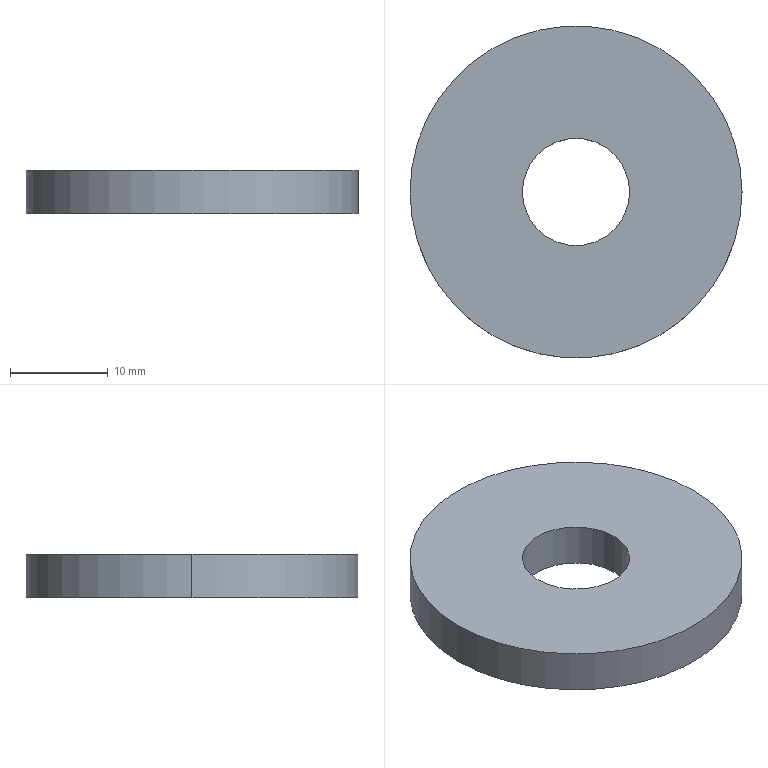Part | STEP file | DCV-000-028 | 1 solid | 6 faces | box 34 x 34 x 4.5 mm | volume 3658 mm3 | cylinder 4 | plane 2 | commonest cylinder face diameters 11 x2 34 x2
STEP:
#1=CARTESIAN_POINT('',(0.,0.,0.));
#2=DIRECTION('',(0.,0.,1.));
#3=DIRECTION('',(1.,0.,0.));
#4=AXIS2_PLACEMENT_3D('',#1,#2,#3);
#5=CARTESIAN_POINT('',(5.5,0.,0.));
#6=VERTEX_POINT('',#5);
#7=CARTESIAN_POINT('',(5.5,0.,4.5));
#8=VERTEX_POINT('',#7);
#9=CARTESIAN_POINT('',(5.5,0.,-43.793));
#10=DIRECTION('',(0.,0.,1.));
#11=VECTOR('',#10,1.);
#12=LINE('',#9,#11);
#13=CARTESIAN_POINT('',(0.,0.,-43.793));
#14=DIRECTION('',(0.,0.,1.));
#15=DIRECTION('',(1.,0.,0.));
#16=AXIS2_PLACEMENT_3D('',#13,#14,#15);
#17=CYLINDRICAL_SURFACE('',#16,5.5);
#18=CARTESIAN_POINT('',(6.283,0.));
#19=DIRECTION('',(0.,1.));
#20=VECTOR('',#19,1.);
#21=LINE('',#18,#20);
#22=(GEOMETRIC_REPRESENTATION_CONTEXT(2)PARAMETRIC_REPRESENTATION_CONTEXT()REPRESENTATION_CONTEXT('',''));
#23=DEFINITIONAL_REPRESENTATION('',(#21),#22);
#24=PCURVE('',#17,#23);
#25=CARTESIAN_POINT('',(0.,0.,-43.793));
#26=DIRECTION('',(0.,0.,1.));
#27=DIRECTION('',(1.,0.,0.));
#28=AXIS2_PLACEMENT_3D('',#25,#26,#27);
#29=CYLINDRICAL_SURFACE('',#28,5.5);
#30=CARTESIAN_POINT('',(0.,0.));
#31=DIRECTION('',(0.,1.));
#32=VECTOR('',#31,1.);
#33=LINE('',#30,#32);
#34=(GEOMETRIC_REPRESENTATION_CONTEXT(2)PARAMETRIC_REPRESENTATION_CONTEXT()REPRESENTATION_CONTEXT('',''));
#35=DEFINITIONAL_REPRESENTATION('',(#33),#34);
#36=PCURVE('',#29,#35);
#37=SURFACE_CURVE('',#12,(#24,#36),.PCURVE_S1.);
#38=EDGE_CURVE('',#6,#8,#37,.T.);
#39=ORIENTED_EDGE('',*,*,#38,.T.);
#40=CARTESIAN_POINT('',(-5.5,0.,4.5));
#41=VERTEX_POINT('',#40);
#42=CARTESIAN_POINT('',(0.,0.,4.5));
#43=DIRECTION('',(0.,0.,-1.));
#44=DIRECTION('',(1.,0.,0.));
#45=AXIS2_PLACEMENT_3D('',#42,#43,#44);
#46=CIRCLE('',#45,5.5);
#47=CARTESIAN_POINT('',(6.283,48.293));
#48=DIRECTION('',(-1.,0.));
#49=VECTOR('',#48,1.);
#50=LINE('',#47,#49);
#51=(GEOMETRIC_REPRESENTATION_CONTEXT(2)PARAMETRIC_REPRESENTATION_CONTEXT()REPRESENTATION_CONTEXT('',''));
#52=DEFINITIONAL_REPRESENTATION('',(#50),#51);
#53=PCURVE('',#17,#52);
#54=CARTESIAN_POINT('',(0.,0.,4.5));
#55=DIRECTION('',(0.,0.,1.));
#56=DIRECTION('',(1.,0.,0.));
#57=AXIS2_PLACEMENT_3D('',#54,#55,#56);
#58=PLANE('',#57);
#59=CARTESIAN_POINT('',(5.5,0.));
#60=CARTESIAN_POINT('',(5.5,-9.526));
#61=CARTESIAN_POINT('',(-2.75,-4.763));
#62=CARTESIAN_POINT('',(-11.,0.));
#63=CARTESIAN_POINT('',(-2.75,4.763));
#64=CARTESIAN_POINT('',(5.5,9.526));
#65=CARTESIAN_POINT('',(5.5,0.));
#66=(BOUNDED_CURVE()B_SPLINE_CURVE(2,(#59,#60,#61,#62,#63,#64,#65),.UNSPECIFIED.,.T.,.F.)B_SPLINE_CURVE_WITH_KNOTS((1,2,2,2,2,1),(-2.094,0.,2.094,4.189,6.283,8.378),.UNSPECIFIED.)CURVE()GEOMETRIC_REPRESENTATION_ITEM()RATIONAL_B_SPLINE_CURVE((1.,0.5,1.,0.5,1.,0.5,1.))REPRESENTATION_ITEM(''));
#67=(GEOMETRIC_REPRESENTATION_CONTEXT(2)PARAMETRIC_REPRESENTATION_CONTEXT()REPRESENTATION_CONTEXT('',''));
#68=DEFINITIONAL_REPRESENTATION('',(#66),#67);
#69=PCURVE('',#58,#68);
#70=SURFACE_CURVE('',#46,(#53,#69),.PCURVE_S1.);
#71=EDGE_CURVE('',#8,#41,#70,.T.);
#72=ORIENTED_EDGE('',*,*,#71,.T.);
#73=CARTESIAN_POINT('',(-5.5,0.,0.));
#74=VERTEX_POINT('',#73);
#75=CARTESIAN_POINT('',(-5.5,0.,-43.793));
#76=DIRECTION('',(0.,0.,1.));
#77=VECTOR('',#76,1.);
#78=LINE('',#75,#77);
#79=CARTESIAN_POINT('',(3.142,0.));
#80=DIRECTION('',(0.,1.));
#81=VECTOR('',#80,1.);
#82=LINE('',#79,#81);
#83=(GEOMETRIC_REPRESENTATION_CONTEXT(2)PARAMETRIC_REPRESENTATION_CONTEXT()REPRESENTATION_CONTEXT('',''));
#84=DEFINITIONAL_REPRESENTATION('',(#82),#83);
#85=PCURVE('',#17,#84);
#86=CARTESIAN_POINT('',(3.142,0.));
#87=DIRECTION('',(0.,1.));
#88=VECTOR('',#87,1.);
#89=LINE('',#86,#88);
#90=(GEOMETRIC_REPRESENTATION_CONTEXT(2)PARAMETRIC_REPRESENTATION_CONTEXT()REPRESENTATION_CONTEXT('',''));
#91=DEFINITIONAL_REPRESENTATION('',(#89),#90);
#92=PCURVE('',#29,#91);
#93=SURFACE_CURVE('',#78,(#85,#92),.PCURVE_S1.);
#94=EDGE_CURVE('',#74,#41,#93,.T.);
#95=ORIENTED_EDGE('',*,*,#94,.F.);
#96=CARTESIAN_POINT('',(0.,0.,0.));
#97=DIRECTION('',(0.,0.,1.));
#98=DIRECTION('',(1.,0.,0.));
#99=AXIS2_PLACEMENT_3D('',#96,#97,#98);
#100=CIRCLE('',#99,5.5);
#101=CARTESIAN_POINT('',(0.,43.793));
#102=DIRECTION('',(1.,0.));
#103=VECTOR('',#102,1.);
#104=LINE('',#101,#103);
#105=(GEOMETRIC_REPRESENTATION_CONTEXT(2)PARAMETRIC_REPRESENTATION_CONTEXT()REPRESENTATION_CONTEXT('',''));
#106=DEFINITIONAL_REPRESENTATION('',(#104),#105);
#107=PCURVE('',#17,#106);
#108=CARTESIAN_POINT('',(0.,0.,0.));
#109=DIRECTION('',(0.,0.,1.));
#110=DIRECTION('',(1.,0.,0.));
#111=AXIS2_PLACEMENT_3D('',#108,#109,#110);
#112=PLANE('',#111);
#113=CARTESIAN_POINT('',(0.,0.));
#114=DIRECTION('',(1.,0.));
#115=AXIS2_PLACEMENT_2D('',#113,#114);
#116=CIRCLE('',#115,5.5);
#117=(GEOMETRIC_REPRESENTATION_CONTEXT(2)PARAMETRIC_REPRESENTATION_CONTEXT()REPRESENTATION_CONTEXT('',''));
#118=DEFINITIONAL_REPRESENTATION('',(#116),#117);
#119=PCURVE('',#112,#118);
#120=SURFACE_CURVE('',#100,(#107,#119),.PCURVE_S1.);
#121=EDGE_CURVE('',#74,#6,#120,.T.);
#122=ORIENTED_EDGE('',*,*,#121,.T.);
#123=EDGE_LOOP('',(#39,#72,#95,#122));
#124=FACE_BOUND('',#123,.F.);
#125=ADVANCED_FACE('',(#124),#17,.F.);
#126=CARTESIAN_POINT('',(17.,0.,0.));
#127=VERTEX_POINT('',#126);
#128=CARTESIAN_POINT('',(-17.,0.,0.));
#129=VERTEX_POINT('',#128);
#130=CARTESIAN_POINT('',(0.,0.,0.));
#131=DIRECTION('',(0.,0.,1.));
#132=DIRECTION('',(1.,0.,0.));
#133=AXIS2_PLACEMENT_3D('',#130,#131,#132);
#134=CIRCLE('',#133,17.);
#135=CARTESIAN_POINT('',(0.,0.,0.));
#136=DIRECTION('',(0.,0.,1.));
#137=DIRECTION('',(1.,0.,0.));
#138=AXIS2_PLACEMENT_3D('',#135,#136,#137);
#139=CYLINDRICAL_SURFACE('',#138,17.);
#140=CARTESIAN_POINT('',(0.,0.));
#141=DIRECTION('',(1.,0.));
#142=VECTOR('',#141,1.);
#143=LINE('',#140,#142);
#144=(GEOMETRIC_REPRESENTATION_CONTEXT(2)PARAMETRIC_REPRESENTATION_CONTEXT()REPRESENTATION_CONTEXT('',''));
#145=DEFINITIONAL_REPRESENTATION('',(#143),#144);
#146=PCURVE('',#139,#145);
#147=CARTESIAN_POINT('',(0.,0.));
#148=DIRECTION('',(1.,0.));
#149=AXIS2_PLACEMENT_2D('',#147,#148);
#150=CIRCLE('',#149,17.);
#151=(GEOMETRIC_REPRESENTATION_CONTEXT(2)PARAMETRIC_REPRESENTATION_CONTEXT()REPRESENTATION_CONTEXT('',''));
#152=DEFINITIONAL_REPRESENTATION('',(#150),#151);
#153=PCURVE('',#112,#152);
#154=SURFACE_CURVE('',#134,(#146,#153),.PCURVE_S1.);
#155=EDGE_CURVE('',#127,#129,#154,.T.);
#156=ORIENTED_EDGE('',*,*,#155,.T.);
#157=CARTESIAN_POINT('',(-17.,0.,4.5));
#158=VERTEX_POINT('',#157);
#159=CARTESIAN_POINT('',(-17.,0.,0.));
#160=DIRECTION('',(0.,0.,1.));
#161=VECTOR('',#160,1.);
#162=LINE('',#159,#161);
#163=CARTESIAN_POINT('',(3.142,0.));
#164=DIRECTION('',(0.,1.));
#165=VECTOR('',#164,1.);
#166=LINE('',#163,#165);
#167=(GEOMETRIC_REPRESENTATION_CONTEXT(2)PARAMETRIC_REPRESENTATION_CONTEXT()REPRESENTATION_CONTEXT('',''));
#168=DEFINITIONAL_REPRESENTATION('',(#166),#167);
#169=PCURVE('',#139,#168);
#170=CARTESIAN_POINT('',(0.,0.,0.));
#171=DIRECTION('',(0.,0.,1.));
#172=DIRECTION('',(1.,0.,0.));
#173=AXIS2_PLACEMENT_3D('',#170,#171,#172);
#174=CYLINDRICAL_SURFACE('',#173,17.);
#175=CARTESIAN_POINT('',(3.142,0.));
#176=DIRECTION('',(0.,1.));
#177=VECTOR('',#176,1.);
#178=LINE('',#175,#177);
#179=(GEOMETRIC_REPRESENTATION_CONTEXT(2)PARAMETRIC_REPRESENTATION_CONTEXT()REPRESENTATION_CONTEXT('',''));
#180=DEFINITIONAL_REPRESENTATION('',(#178),#179);
#181=PCURVE('',#174,#180);
#182=SURFACE_CURVE('',#162,(#169,#181),.PCURVE_S1.);
#183=EDGE_CURVE('',#129,#158,#182,.T.);
#184=ORIENTED_EDGE('',*,*,#183,.T.);
#185=CARTESIAN_POINT('',(17.,0.,4.5));
#186=VERTEX_POINT('',#185);
#187=CARTESIAN_POINT('',(0.,0.,4.5));
#188=DIRECTION('',(0.,0.,1.));
#189=DIRECTION('',(1.,0.,0.));
#190=AXIS2_PLACEMENT_3D('',#187,#188,#189);
#191=CIRCLE('',#190,17.);
#192=CARTESIAN_POINT('',(0.,4.5));
#193=DIRECTION('',(1.,0.));
#194=VECTOR('',#193,1.);
#195=LINE('',#192,#194);
#196=(GEOMETRIC_REPRESENTATION_CONTEXT(2)PARAMETRIC_REPRESENTATION_CONTEXT()REPRESENTATION_CONTEXT('',''));
#197=DEFINITIONAL_REPRESENTATION('',(#195),#196);
#198=PCURVE('',#139,#197);
#199=CARTESIAN_POINT('',(0.,0.));
#200=DIRECTION('',(1.,0.));
#201=AXIS2_PLACEMENT_2D('',#199,#200);
#202=CIRCLE('',#201,17.);
#203=(GEOMETRIC_REPRESENTATION_CONTEXT(2)PARAMETRIC_REPRESENTATION_CONTEXT()REPRESENTATION_CONTEXT('',''));
#204=DEFINITIONAL_REPRESENTATION('',(#202),#203);
#205=PCURVE('',#58,#204);
#206=SURFACE_CURVE('',#191,(#198,#205),.PCURVE_S1.);
#207=EDGE_CURVE('',#186,#158,#206,.T.);
#208=ORIENTED_EDGE('',*,*,#207,.F.);
#209=CARTESIAN_POINT('',(17.,0.,0.));
#210=DIRECTION('',(0.,0.,1.));
#211=VECTOR('',#210,1.);
#212=LINE('',#209,#211);
#213=CARTESIAN_POINT('',(0.,0.));
#214=DIRECTION('',(0.,1.));
#215=VECTOR('',#214,1.);
#216=LINE('',#213,#215);
#217=(GEOMETRIC_REPRESENTATION_CONTEXT(2)PARAMETRIC_REPRESENTATION_CONTEXT()REPRESENTATION_CONTEXT('',''));
#218=DEFINITIONAL_REPRESENTATION('',(#216),#217);
#219=PCURVE('',#139,#218);
#220=CARTESIAN_POINT('',(6.283,0.));
#221=DIRECTION('',(0.,1.));
#222=VECTOR('',#221,1.);
#223=LINE('',#220,#222);
#224=(GEOMETRIC_REPRESENTATION_CONTEXT(2)PARAMETRIC_REPRESENTATION_CONTEXT()REPRESENTATION_CONTEXT('',''));
#225=DEFINITIONAL_REPRESENTATION('',(#223),#224);
#226=PCURVE('',#174,#225);
#227=SURFACE_CURVE('',#212,(#219,#226),.PCURVE_S1.);
#228=EDGE_CURVE('',#127,#186,#227,.T.);
#229=ORIENTED_EDGE('',*,*,#228,.F.);
#230=EDGE_LOOP('',(#156,#184,#208,#229));
#231=FACE_BOUND('',#230,.T.);
#232=ADVANCED_FACE('',(#231),#139,.T.);
#233=CARTESIAN_POINT('',(0.,0.,0.));
#234=DIRECTION('',(0.,0.,1.));
#235=DIRECTION('',(1.,0.,0.));
#236=AXIS2_PLACEMENT_3D('',#233,#234,#235);
#237=CIRCLE('',#236,5.5);
#238=CARTESIAN_POINT('',(0.,0.));
#239=DIRECTION('',(1.,0.));
#240=AXIS2_PLACEMENT_2D('',#238,#239);
#241=CIRCLE('',#240,5.5);
#242=(GEOMETRIC_REPRESENTATION_CONTEXT(2)PARAMETRIC_REPRESENTATION_CONTEXT()REPRESENTATION_CONTEXT('',''));
#243=DEFINITIONAL_REPRESENTATION('',(#241),#242);
#244=PCURVE('',#112,#243);
#245=CARTESIAN_POINT('',(0.,43.793));
#246=DIRECTION('',(1.,0.));
#247=VECTOR('',#246,1.);
#248=LINE('',#245,#247);
#249=(GEOMETRIC_REPRESENTATION_CONTEXT(2)PARAMETRIC_REPRESENTATION_CONTEXT()REPRESENTATION_CONTEXT('',''));
#250=DEFINITIONAL_REPRESENTATION('',(#248),#249);
#251=PCURVE('',#29,#250);
#252=SURFACE_CURVE('',#237,(#244,#251),.PCURVE_S1.);
#253=EDGE_CURVE('',#6,#74,#252,.T.);
#254=ORIENTED_EDGE('',*,*,#253,.T.);
#255=ORIENTED_EDGE('',*,*,#121,.T.);
#256=EDGE_LOOP('',(#254,#255));
#257=FACE_BOUND('',#256,.T.);
#258=ORIENTED_EDGE('',*,*,#155,.F.);
#259=CARTESIAN_POINT('',(0.,0.,0.));
#260=DIRECTION('',(0.,0.,1.));
#261=DIRECTION('',(1.,0.,0.));
#262=AXIS2_PLACEMENT_3D('',#259,#260,#261);
#263=CIRCLE('',#262,17.);
#264=CARTESIAN_POINT('',(0.,0.));
#265=DIRECTION('',(1.,0.));
#266=AXIS2_PLACEMENT_2D('',#264,#265);
#267=CIRCLE('',#266,17.);
#268=(GEOMETRIC_REPRESENTATION_CONTEXT(2)PARAMETRIC_REPRESENTATION_CONTEXT()REPRESENTATION_CONTEXT('',''));
#269=DEFINITIONAL_REPRESENTATION('',(#267),#268);
#270=PCURVE('',#112,#269);
#271=CARTESIAN_POINT('',(0.,0.));
#272=DIRECTION('',(1.,0.));
#273=VECTOR('',#272,1.);
#274=LINE('',#271,#273);
#275=(GEOMETRIC_REPRESENTATION_CONTEXT(2)PARAMETRIC_REPRESENTATION_CONTEXT()REPRESENTATION_CONTEXT('',''));
#276=DEFINITIONAL_REPRESENTATION('',(#274),#275);
#277=PCURVE('',#174,#276);
#278=SURFACE_CURVE('',#263,(#270,#277),.PCURVE_S1.);
#279=EDGE_CURVE('',#129,#127,#278,.T.);
#280=ORIENTED_EDGE('',*,*,#279,.F.);
#281=EDGE_LOOP('',(#258,#280));
#282=FACE_BOUND('',#281,.T.);
#283=ADVANCED_FACE('',(#257,#282),#112,.F.);
#284=ORIENTED_EDGE('',*,*,#71,.T.);
#285=CARTESIAN_POINT('',(0.,0.,4.5));
#286=DIRECTION('',(0.,0.,-1.));
#287=DIRECTION('',(1.,0.,0.));
#288=AXIS2_PLACEMENT_3D('',#285,#286,#287);
#289=CIRCLE('',#288,5.5);
#290=CARTESIAN_POINT('',(5.5,0.));
#291=CARTESIAN_POINT('',(5.5,-9.526));
#292=CARTESIAN_POINT('',(-2.75,-4.763));
#293=CARTESIAN_POINT('',(-11.,0.));
#294=CARTESIAN_POINT('',(-2.75,4.763));
#295=CARTESIAN_POINT('',(5.5,9.526));
#296=CARTESIAN_POINT('',(5.5,0.));
#297=(BOUNDED_CURVE()B_SPLINE_CURVE(2,(#290,#291,#292,#293,#294,#295,#296),.UNSPECIFIED.,.T.,.F.)B_SPLINE_CURVE_WITH_KNOTS((1,2,2,2,2,1),(-2.094,0.,2.094,4.189,6.283,8.378),.UNSPECIFIED.)CURVE()GEOMETRIC_REPRESENTATION_ITEM()RATIONAL_B_SPLINE_CURVE((1.,0.5,1.,0.5,1.,0.5,1.))REPRESENTATION_ITEM(''));
#298=(GEOMETRIC_REPRESENTATION_CONTEXT(2)PARAMETRIC_REPRESENTATION_CONTEXT()REPRESENTATION_CONTEXT('',''));
#299=DEFINITIONAL_REPRESENTATION('',(#297),#298);
#300=PCURVE('',#58,#299);
#301=CARTESIAN_POINT('',(6.283,48.293));
#302=DIRECTION('',(-1.,0.));
#303=VECTOR('',#302,1.);
#304=LINE('',#301,#303);
#305=(GEOMETRIC_REPRESENTATION_CONTEXT(2)PARAMETRIC_REPRESENTATION_CONTEXT()REPRESENTATION_CONTEXT('',''));
#306=DEFINITIONAL_REPRESENTATION('',(#304),#305);
#307=PCURVE('',#29,#306);
#308=SURFACE_CURVE('',#289,(#300,#307),.PCURVE_S1.);
#309=EDGE_CURVE('',#41,#8,#308,.T.);
#310=ORIENTED_EDGE('',*,*,#309,.T.);
#311=EDGE_LOOP('',(#284,#310));
#312=FACE_BOUND('',#311,.T.);
#313=ORIENTED_EDGE('',*,*,#207,.T.);
#314=CARTESIAN_POINT('',(0.,0.,4.5));
#315=DIRECTION('',(0.,0.,1.));
#316=DIRECTION('',(1.,0.,0.));
#317=AXIS2_PLACEMENT_3D('',#314,#315,#316);
#318=CIRCLE('',#317,17.);
#319=CARTESIAN_POINT('',(0.,0.));
#320=DIRECTION('',(1.,0.));
#321=AXIS2_PLACEMENT_2D('',#319,#320);
#322=CIRCLE('',#321,17.);
#323=(GEOMETRIC_REPRESENTATION_CONTEXT(2)PARAMETRIC_REPRESENTATION_CONTEXT()REPRESENTATION_CONTEXT('',''));
#324=DEFINITIONAL_REPRESENTATION('',(#322),#323);
#325=PCURVE('',#58,#324);
#326=CARTESIAN_POINT('',(0.,4.5));
#327=DIRECTION('',(1.,0.));
#328=VECTOR('',#327,1.);
#329=LINE('',#326,#328);
#330=(GEOMETRIC_REPRESENTATION_CONTEXT(2)PARAMETRIC_REPRESENTATION_CONTEXT()REPRESENTATION_CONTEXT('',''));
#331=DEFINITIONAL_REPRESENTATION('',(#329),#330);
#332=PCURVE('',#174,#331);
#333=SURFACE_CURVE('',#318,(#325,#332),.PCURVE_S1.);
#334=EDGE_CURVE('',#158,#186,#333,.T.);
#335=ORIENTED_EDGE('',*,*,#334,.T.);
#336=EDGE_LOOP('',(#313,#335));
#337=FACE_BOUND('',#336,.T.);
#338=ADVANCED_FACE('',(#312,#337),#58,.T.);
#339=ORIENTED_EDGE('',*,*,#183,.F.);
#340=ORIENTED_EDGE('',*,*,#279,.T.);
#341=ORIENTED_EDGE('',*,*,#228,.T.);
#342=ORIENTED_EDGE('',*,*,#334,.F.);
#343=EDGE_LOOP('',(#339,#340,#341,#342));
#344=FACE_BOUND('',#343,.T.);
#345=ADVANCED_FACE('',(#344),#174,.T.);
#346=ORIENTED_EDGE('',*,*,#309,.T.);
#347=ORIENTED_EDGE('',*,*,#38,.F.);
#348=ORIENTED_EDGE('',*,*,#253,.T.);
#349=ORIENTED_EDGE('',*,*,#94,.T.);
#350=EDGE_LOOP('',(#346,#347,#348,#349));
#351=FACE_BOUND('',#350,.F.);
#352=ADVANCED_FACE('',(#351),#29,.F.);
#353=CLOSED_SHELL('',(#125,#232,#283,#338,#345,#352));
#354=MANIFOLD_SOLID_BREP('',#353);
#355=(LENGTH_UNIT()NAMED_UNIT(*)SI_UNIT(.MILLI.,.METRE.));
#356=UNCERTAINTY_MEASURE_WITH_UNIT(LENGTH_MEASURE(0.0000001),#355,'','');
#357=(NAMED_UNIT(*)PLANE_ANGLE_UNIT()SI_UNIT($,.RADIAN.));
#358=(NAMED_UNIT(*)SI_UNIT($,.STERADIAN.)SOLID_ANGLE_UNIT());
#359=(GEOMETRIC_REPRESENTATION_CONTEXT(3)GLOBAL_UNCERTAINTY_ASSIGNED_CONTEXT((#356))GLOBAL_UNIT_ASSIGNED_CONTEXT((#355,#357,#358))REPRESENTATION_CONTEXT('',''));
#360=ADVANCED_BREP_SHAPE_REPRESENTATION('',(#4,#354),#359);